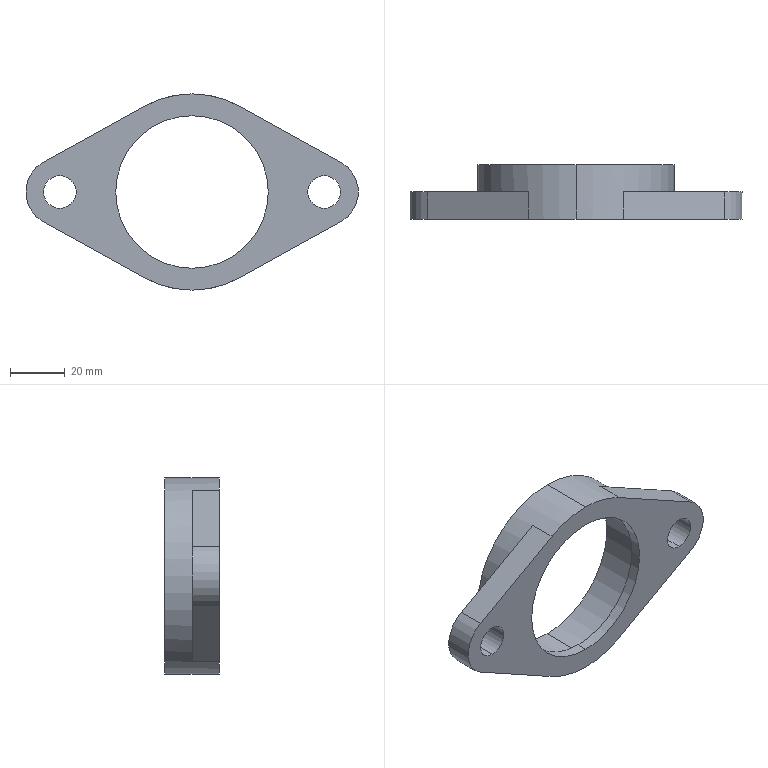Part | SolidWorks | features ICE 3, Extrusion 1 | 1 solid | 21 faces | box 122 x 20 x 72 mm | volume 37889 mm3 | cylinder 12 | plane 9 | commonest cylinder face diameters 12 x4 25 x2 56 x2 62 x2 72 x2
STEP:
#1=CARTESIAN_POINT('',(0.,0.,-28.));
#2=VERTEX_POINT('',#1);
#3=CARTESIAN_POINT('',(0.,0.,28.));
#4=VERTEX_POINT('',#3);
#5=CARTESIAN_POINT('',(0.,0.,0.));
#6=DIRECTION('',(0.,1.,0.));
#7=DIRECTION('',(0.,0.,1.));
#8=AXIS2_PLACEMENT_3D('',#5,#6,#7);
#9=CIRCLE('',#8,28.);
#10=EDGE_CURVE('',#2,#4,#9,.T.);
#11=ORIENTED_EDGE('',*,*,#10,.F.);
#12=CARTESIAN_POINT('',(0.,4.,-28.));
#13=VERTEX_POINT('',#12);
#14=CARTESIAN_POINT('',(0.,-12.,-28.));
#15=DIRECTION('',(0.,1.,0.));
#16=VECTOR('',#15,1000.);
#17=LINE('',#14,#16);
#18=EDGE_CURVE('',#2,#13,#17,.T.);
#19=ORIENTED_EDGE('',*,*,#18,.T.);
#20=CARTESIAN_POINT('',(0.,4.,28.));
#21=VERTEX_POINT('',#20);
#22=CARTESIAN_POINT('',(0.,4.,0.));
#23=DIRECTION('',(0.,1.,0.));
#24=DIRECTION('',(0.,0.,1.));
#25=AXIS2_PLACEMENT_3D('',#22,#23,#24);
#26=CIRCLE('',#25,28.);
#27=EDGE_CURVE('',#13,#21,#26,.T.);
#28=ORIENTED_EDGE('',*,*,#27,.T.);
#29=CARTESIAN_POINT('',(0.,-12.,28.));
#30=DIRECTION('',(0.,1.,0.));
#31=VECTOR('',#30,1000.);
#32=LINE('',#29,#31);
#33=EDGE_CURVE('',#4,#21,#32,.T.);
#34=ORIENTED_EDGE('',*,*,#33,.F.);
#35=EDGE_LOOP('',(#11,#19,#28,#34));
#36=FACE_OUTER_BOUND('',#35,.T.);
#37=CARTESIAN_POINT('',(0.,-12.,0.));
#38=DIRECTION('',(0.,1.,0.));
#39=DIRECTION('',(0.,0.,1.));
#40=AXIS2_PLACEMENT_3D('',#37,#38,#39);
#41=CYLINDRICAL_SURFACE('',#40,28.);
#42=ADVANCED_FACE('',(#36),#41,.F.);
#43=CARTESIAN_POINT('',(0.,4.,-31.));
#44=VERTEX_POINT('',#43);
#45=CARTESIAN_POINT('',(0.,4.,31.));
#46=VERTEX_POINT('',#45);
#47=CARTESIAN_POINT('',(0.,4.,0.));
#48=DIRECTION('',(0.,1.,0.));
#49=DIRECTION('',(0.,0.,1.));
#50=AXIS2_PLACEMENT_3D('',#47,#48,#49);
#51=CIRCLE('',#50,31.);
#52=EDGE_CURVE('',#44,#46,#51,.T.);
#53=ORIENTED_EDGE('',*,*,#52,.F.);
#54=CARTESIAN_POINT('',(0.,20.,-31.));
#55=VERTEX_POINT('',#54);
#56=CARTESIAN_POINT('',(0.,4.,-31.));
#57=DIRECTION('',(0.,1.,0.));
#58=VECTOR('',#57,1000.);
#59=LINE('',#56,#58);
#60=EDGE_CURVE('',#44,#55,#59,.T.);
#61=ORIENTED_EDGE('',*,*,#60,.T.);
#62=CARTESIAN_POINT('',(0.,20.,31.));
#63=VERTEX_POINT('',#62);
#64=CARTESIAN_POINT('',(0.,20.,0.));
#65=DIRECTION('',(0.,1.,0.));
#66=DIRECTION('',(0.,0.,1.));
#67=AXIS2_PLACEMENT_3D('',#64,#65,#66);
#68=CIRCLE('',#67,31.);
#69=EDGE_CURVE('',#55,#63,#68,.T.);
#70=ORIENTED_EDGE('',*,*,#69,.T.);
#71=CARTESIAN_POINT('',(0.,4.,31.));
#72=DIRECTION('',(0.,1.,0.));
#73=VECTOR('',#72,1000.);
#74=LINE('',#71,#73);
#75=EDGE_CURVE('',#46,#63,#74,.T.);
#76=ORIENTED_EDGE('',*,*,#75,.F.);
#77=EDGE_LOOP('',(#53,#61,#70,#76));
#78=FACE_OUTER_BOUND('',#77,.T.);
#79=CARTESIAN_POINT('',(0.,4.,0.));
#80=DIRECTION('',(0.,1.,0.));
#81=DIRECTION('',(0.,0.,1.));
#82=AXIS2_PLACEMENT_3D('',#79,#80,#81);
#83=CYLINDRICAL_SURFACE('',#82,31.);
#84=ADVANCED_FACE('',(#78),#83,.F.);
#85=CARTESIAN_POINT('',(-48.5,10.,-6.));
#86=VERTEX_POINT('',#85);
#87=CARTESIAN_POINT('',(-48.5,10.,6.));
#88=VERTEX_POINT('',#87);
#89=CARTESIAN_POINT('',(-48.5,10.,0.));
#90=DIRECTION('',(0.,1.,0.));
#91=DIRECTION('',(0.,0.,1.));
#92=AXIS2_PLACEMENT_3D('',#89,#90,#91);
#93=CIRCLE('',#92,6.);
#94=EDGE_CURVE('',#86,#88,#93,.T.);
#95=ORIENTED_EDGE('',*,*,#94,.T.);
#96=CARTESIAN_POINT('',(-48.5,0.,6.));
#97=VERTEX_POINT('',#96);
#98=CARTESIAN_POINT('',(-48.5,10.,6.));
#99=DIRECTION('',(0.,-1.,0.));
#100=VECTOR('',#99,1000.);
#101=LINE('',#98,#100);
#102=EDGE_CURVE('',#88,#97,#101,.T.);
#103=ORIENTED_EDGE('',*,*,#102,.T.);
#104=CARTESIAN_POINT('',(-48.5,0.,-6.));
#105=VERTEX_POINT('',#104);
#106=CARTESIAN_POINT('',(-48.5,0.,0.));
#107=DIRECTION('',(0.,1.,0.));
#108=DIRECTION('',(0.,0.,1.));
#109=AXIS2_PLACEMENT_3D('',#106,#107,#108);
#110=CIRCLE('',#109,6.);
#111=EDGE_CURVE('',#105,#97,#110,.T.);
#112=ORIENTED_EDGE('',*,*,#111,.F.);
#113=CARTESIAN_POINT('',(-48.5,10.,-6.));
#114=DIRECTION('',(0.,-1.,0.));
#115=VECTOR('',#114,1000.);
#116=LINE('',#113,#115);
#117=EDGE_CURVE('',#86,#105,#116,.T.);
#118=ORIENTED_EDGE('',*,*,#117,.F.);
#119=EDGE_LOOP('',(#95,#103,#112,#118));
#120=FACE_OUTER_BOUND('',#119,.T.);
#121=CARTESIAN_POINT('',(-48.5,10.,0.));
#122=DIRECTION('',(0.,-1.,0.));
#123=DIRECTION('',(0.,0.,-1.));
#124=AXIS2_PLACEMENT_3D('',#121,#122,#123);
#125=CYLINDRICAL_SURFACE('',#124,6.);
#126=ADVANCED_FACE('',(#120),#125,.F.);
#127=CARTESIAN_POINT('',(48.5,10.,-6.));
#128=VERTEX_POINT('',#127);
#129=CARTESIAN_POINT('',(48.5,10.,6.));
#130=VERTEX_POINT('',#129);
#131=CARTESIAN_POINT('',(48.5,10.,0.));
#132=DIRECTION('',(0.,1.,0.));
#133=DIRECTION('',(0.,0.,1.));
#134=AXIS2_PLACEMENT_3D('',#131,#132,#133);
#135=CIRCLE('',#134,6.);
#136=EDGE_CURVE('',#128,#130,#135,.T.);
#137=ORIENTED_EDGE('',*,*,#136,.T.);
#138=CARTESIAN_POINT('',(48.5,0.,6.));
#139=VERTEX_POINT('',#138);
#140=CARTESIAN_POINT('',(48.5,10.,6.));
#141=DIRECTION('',(0.,-1.,0.));
#142=VECTOR('',#141,1000.);
#143=LINE('',#140,#142);
#144=EDGE_CURVE('',#130,#139,#143,.T.);
#145=ORIENTED_EDGE('',*,*,#144,.T.);
#146=CARTESIAN_POINT('',(48.5,0.,-6.));
#147=VERTEX_POINT('',#146);
#148=CARTESIAN_POINT('',(48.5,0.,0.));
#149=DIRECTION('',(0.,1.,0.));
#150=DIRECTION('',(0.,0.,1.));
#151=AXIS2_PLACEMENT_3D('',#148,#149,#150);
#152=CIRCLE('',#151,6.);
#153=EDGE_CURVE('',#147,#139,#152,.T.);
#154=ORIENTED_EDGE('',*,*,#153,.F.);
#155=CARTESIAN_POINT('',(48.5,10.,-6.));
#156=DIRECTION('',(0.,-1.,0.));
#157=VECTOR('',#156,1000.);
#158=LINE('',#155,#157);
#159=EDGE_CURVE('',#128,#147,#158,.T.);
#160=ORIENTED_EDGE('',*,*,#159,.F.);
#161=EDGE_LOOP('',(#137,#145,#154,#160));
#162=FACE_OUTER_BOUND('',#161,.T.);
#163=CARTESIAN_POINT('',(48.5,10.,0.));
#164=DIRECTION('',(0.,-1.,0.));
#165=DIRECTION('',(0.,0.,-1.));
#166=AXIS2_PLACEMENT_3D('',#163,#164,#165);
#167=CYLINDRICAL_SURFACE('',#166,6.);
#168=ADVANCED_FACE('',(#162),#167,.F.);
#169=CARTESIAN_POINT('',(0.,20.,36.));
#170=VERTEX_POINT('',#169);
#171=CARTESIAN_POINT('',(0.,20.,-36.));
#172=VERTEX_POINT('',#171);
#173=CARTESIAN_POINT('',(0.,20.,0.));
#174=DIRECTION('',(0.,1.,0.));
#175=DIRECTION('',(0.,0.,1.));
#176=AXIS2_PLACEMENT_3D('',#173,#174,#175);
#177=CIRCLE('',#176,36.);
#178=EDGE_CURVE('',#170,#172,#177,.T.);
#179=ORIENTED_EDGE('',*,*,#178,.F.);
#180=CARTESIAN_POINT('',(0.,0.,36.));
#181=VERTEX_POINT('',#180);
#182=CARTESIAN_POINT('',(0.,10.,36.));
#183=DIRECTION('',(0.,-1.,0.));
#184=VECTOR('',#183,1000.);
#185=LINE('',#182,#184);
#186=EDGE_CURVE('',#170,#181,#185,.T.);
#187=ORIENTED_EDGE('',*,*,#186,.T.);
#188=CARTESIAN_POINT('',(17.443,0.,31.492));
#189=VERTEX_POINT('',#188);
#190=CARTESIAN_POINT('',(0.,0.,0.));
#191=DIRECTION('',(0.,1.,0.));
#192=DIRECTION('',(0.,0.,1.));
#193=AXIS2_PLACEMENT_3D('',#190,#191,#192);
#194=CIRCLE('',#193,36.);
#195=EDGE_CURVE('',#181,#189,#194,.T.);
#196=ORIENTED_EDGE('',*,*,#195,.T.);
#197=CARTESIAN_POINT('',(17.443,10.,31.492));
#198=VERTEX_POINT('',#197);
#199=CARTESIAN_POINT('',(17.443,10.,31.492));
#200=DIRECTION('',(0.,-1.,0.));
#201=VECTOR('',#200,1000.);
#202=LINE('',#199,#201);
#203=EDGE_CURVE('',#198,#189,#202,.T.);
#204=ORIENTED_EDGE('',*,*,#203,.F.);
#205=CARTESIAN_POINT('',(17.443,10.,-31.492));
#206=VERTEX_POINT('',#205);
#207=CARTESIAN_POINT('',(0.,10.,0.));
#208=DIRECTION('',(0.,1.,0.));
#209=DIRECTION('',(0.,0.,1.));
#210=AXIS2_PLACEMENT_3D('',#207,#208,#209);
#211=CIRCLE('',#210,36.);
#212=EDGE_CURVE('',#198,#206,#211,.T.);
#213=ORIENTED_EDGE('',*,*,#212,.T.);
#214=CARTESIAN_POINT('',(17.443,0.,-31.492));
#215=VERTEX_POINT('',#214);
#216=CARTESIAN_POINT('',(17.443,10.,-31.492));
#217=DIRECTION('',(0.,-1.,0.));
#218=VECTOR('',#217,1000.);
#219=LINE('',#216,#218);
#220=EDGE_CURVE('',#206,#215,#219,.T.);
#221=ORIENTED_EDGE('',*,*,#220,.T.);
#222=CARTESIAN_POINT('',(0.,0.,-36.));
#223=VERTEX_POINT('',#222);
#224=CARTESIAN_POINT('',(0.,0.,0.));
#225=DIRECTION('',(0.,1.,0.));
#226=DIRECTION('',(0.,0.,1.));
#227=AXIS2_PLACEMENT_3D('',#224,#225,#226);
#228=CIRCLE('',#227,36.);
#229=EDGE_CURVE('',#215,#223,#228,.T.);
#230=ORIENTED_EDGE('',*,*,#229,.T.);
#231=CARTESIAN_POINT('',(0.,10.,-36.));
#232=DIRECTION('',(0.,-1.,0.));
#233=VECTOR('',#232,1000.);
#234=LINE('',#231,#233);
#235=EDGE_CURVE('',#172,#223,#234,.T.);
#236=ORIENTED_EDGE('',*,*,#235,.F.);
#237=EDGE_LOOP('',(#179,#187,#196,#204,#213,#221,#230,#236));
#238=FACE_OUTER_BOUND('',#237,.T.);
#239=CARTESIAN_POINT('',(0.,10.,0.));
#240=DIRECTION('',(0.,-1.,0.));
#241=DIRECTION('',(0.,0.,-1.));
#242=AXIS2_PLACEMENT_3D('',#239,#240,#241);
#243=CYLINDRICAL_SURFACE('',#242,36.);
#244=ADVANCED_FACE('',(#238),#243,.T.);
#245=ORIENTED_EDGE('',*,*,#212,.F.);
#246=CARTESIAN_POINT('',(54.557,10.,10.935));
#247=VERTEX_POINT('',#246);
#248=CARTESIAN_POINT('',(54.557,10.,10.935));
#249=DIRECTION('',(0.8748,0.,-0.4845));
#250=VECTOR('',#249,1000.);
#251=LINE('',#248,#250);
#252=EDGE_CURVE('',#198,#247,#251,.T.);
#253=ORIENTED_EDGE('',*,*,#252,.T.);
#254=CARTESIAN_POINT('',(54.557,10.,-10.935));
#255=VERTEX_POINT('',#254);
#256=CARTESIAN_POINT('',(48.5,10.,0.));
#257=DIRECTION('',(0.,1.,0.));
#258=DIRECTION('',(0.,0.,1.));
#259=AXIS2_PLACEMENT_3D('',#256,#257,#258);
#260=CIRCLE('',#259,12.5);
#261=EDGE_CURVE('',#247,#255,#260,.T.);
#262=ORIENTED_EDGE('',*,*,#261,.T.);
#263=CARTESIAN_POINT('',(17.443,10.,-31.492));
#264=DIRECTION('',(-0.8748,0.,-0.4845));
#265=VECTOR('',#264,1000.);
#266=LINE('',#263,#265);
#267=EDGE_CURVE('',#255,#206,#266,.T.);
#268=ORIENTED_EDGE('',*,*,#267,.T.);
#269=EDGE_LOOP('',(#245,#253,#262,#268));
#270=FACE_OUTER_BOUND('',#269,.T.);
#271=ORIENTED_EDGE('',*,*,#136,.F.);
#272=CARTESIAN_POINT('',(48.5,10.,0.));
#273=DIRECTION('',(0.,1.,0.));
#274=DIRECTION('',(0.,0.,1.));
#275=AXIS2_PLACEMENT_3D('',#272,#273,#274);
#276=CIRCLE('',#275,6.);
#277=EDGE_CURVE('',#130,#128,#276,.T.);
#278=ORIENTED_EDGE('',*,*,#277,.F.);
#279=EDGE_LOOP('',(#271,#278));
#280=FACE_BOUND('',#279,.T.);
#281=CARTESIAN_POINT('',(-48.5,10.,0.));
#282=DIRECTION('',(0.,1.,0.));
#283=DIRECTION('',(0.,0.,1.));
#284=AXIS2_PLACEMENT_3D('',#281,#282,#283);
#285=PLANE('',#284);
#286=ADVANCED_FACE('',(#270,#280),#285,.T.);
#287=CARTESIAN_POINT('',(-17.443,10.,-31.492));
#288=VERTEX_POINT('',#287);
#289=CARTESIAN_POINT('',(-17.443,10.,31.492));
#290=VERTEX_POINT('',#289);
#291=CARTESIAN_POINT('',(0.,10.,0.));
#292=DIRECTION('',(0.,1.,0.));
#293=DIRECTION('',(0.,0.,1.));
#294=AXIS2_PLACEMENT_3D('',#291,#292,#293);
#295=CIRCLE('',#294,36.);
#296=EDGE_CURVE('',#288,#290,#295,.T.);
#297=ORIENTED_EDGE('',*,*,#296,.F.);
#298=CARTESIAN_POINT('',(-54.557,10.,-10.935));
#299=VERTEX_POINT('',#298);
#300=CARTESIAN_POINT('',(-54.557,10.,-10.935));
#301=DIRECTION('',(-0.8748,0.,0.4845));
#302=VECTOR('',#301,1000.);
#303=LINE('',#300,#302);
#304=EDGE_CURVE('',#288,#299,#303,.T.);
#305=ORIENTED_EDGE('',*,*,#304,.T.);
#306=CARTESIAN_POINT('',(-54.557,10.,10.935));
#307=VERTEX_POINT('',#306);
#308=CARTESIAN_POINT('',(-48.5,10.,0.));
#309=DIRECTION('',(0.,1.,0.));
#310=DIRECTION('',(0.,0.,1.));
#311=AXIS2_PLACEMENT_3D('',#308,#309,#310);
#312=CIRCLE('',#311,12.5);
#313=EDGE_CURVE('',#299,#307,#312,.T.);
#314=ORIENTED_EDGE('',*,*,#313,.T.);
#315=CARTESIAN_POINT('',(-17.443,10.,31.492));
#316=DIRECTION('',(0.8748,0.,0.4845));
#317=VECTOR('',#316,1000.);
#318=LINE('',#315,#317);
#319=EDGE_CURVE('',#307,#290,#318,.T.);
#320=ORIENTED_EDGE('',*,*,#319,.T.);
#321=EDGE_LOOP('',(#297,#305,#314,#320));
#322=FACE_OUTER_BOUND('',#321,.T.);
#323=ORIENTED_EDGE('',*,*,#94,.F.);
#324=CARTESIAN_POINT('',(-48.5,10.,0.));
#325=DIRECTION('',(0.,1.,0.));
#326=DIRECTION('',(0.,0.,1.));
#327=AXIS2_PLACEMENT_3D('',#324,#325,#326);
#328=CIRCLE('',#327,6.);
#329=EDGE_CURVE('',#88,#86,#328,.T.);
#330=ORIENTED_EDGE('',*,*,#329,.F.);
#331=EDGE_LOOP('',(#323,#330));
#332=FACE_BOUND('',#331,.T.);
#333=CARTESIAN_POINT('',(-48.5,10.,0.));
#334=DIRECTION('',(0.,1.,0.));
#335=DIRECTION('',(0.,0.,1.));
#336=AXIS2_PLACEMENT_3D('',#333,#334,#335);
#337=PLANE('',#336);
#338=ADVANCED_FACE('',(#322,#332),#337,.T.);
#339=CARTESIAN_POINT('',(0.,0.,0.));
#340=DIRECTION('',(0.,1.,0.));
#341=DIRECTION('',(0.,0.,1.));
#342=AXIS2_PLACEMENT_3D('',#339,#340,#341);
#343=CIRCLE('',#342,28.);
#344=EDGE_CURVE('',#4,#2,#343,.T.);
#345=ORIENTED_EDGE('',*,*,#344,.T.);
#346=ORIENTED_EDGE('',*,*,#10,.T.);
#347=EDGE_LOOP('',(#345,#346));
#348=FACE_BOUND('',#347,.T.);
#349=ORIENTED_EDGE('',*,*,#153,.T.);
#350=CARTESIAN_POINT('',(48.5,0.,0.));
#351=DIRECTION('',(0.,1.,0.));
#352=DIRECTION('',(0.,0.,1.));
#353=AXIS2_PLACEMENT_3D('',#350,#351,#352);
#354=CIRCLE('',#353,6.);
#355=EDGE_CURVE('',#139,#147,#354,.T.);
#356=ORIENTED_EDGE('',*,*,#355,.T.);
#357=EDGE_LOOP('',(#349,#356));
#358=FACE_BOUND('',#357,.T.);
#359=CARTESIAN_POINT('',(-54.557,0.,-10.935));
#360=VERTEX_POINT('',#359);
#361=CARTESIAN_POINT('',(-54.557,0.,10.935));
#362=VERTEX_POINT('',#361);
#363=CARTESIAN_POINT('',(-48.5,0.,0.));
#364=DIRECTION('',(0.,1.,0.));
#365=DIRECTION('',(0.,0.,1.));
#366=AXIS2_PLACEMENT_3D('',#363,#364,#365);
#367=CIRCLE('',#366,12.5);
#368=EDGE_CURVE('',#360,#362,#367,.T.);
#369=ORIENTED_EDGE('',*,*,#368,.F.);
#370=CARTESIAN_POINT('',(-17.443,0.,-31.492));
#371=VERTEX_POINT('',#370);
#372=CARTESIAN_POINT('',(-54.557,0.,-10.935));
#373=DIRECTION('',(-0.8748,0.,0.4845));
#374=VECTOR('',#373,1000.);
#375=LINE('',#372,#374);
#376=EDGE_CURVE('',#371,#360,#375,.T.);
#377=ORIENTED_EDGE('',*,*,#376,.F.);
#378=CARTESIAN_POINT('',(0.,0.,0.));
#379=DIRECTION('',(0.,1.,0.));
#380=DIRECTION('',(0.,0.,1.));
#381=AXIS2_PLACEMENT_3D('',#378,#379,#380);
#382=CIRCLE('',#381,36.);
#383=EDGE_CURVE('',#223,#371,#382,.T.);
#384=ORIENTED_EDGE('',*,*,#383,.F.);
#385=ORIENTED_EDGE('',*,*,#229,.F.);
#386=CARTESIAN_POINT('',(54.557,0.,-10.935));
#387=VERTEX_POINT('',#386);
#388=CARTESIAN_POINT('',(17.443,0.,-31.492));
#389=DIRECTION('',(-0.8748,0.,-0.4845));
#390=VECTOR('',#389,1000.);
#391=LINE('',#388,#390);
#392=EDGE_CURVE('',#387,#215,#391,.T.);
#393=ORIENTED_EDGE('',*,*,#392,.F.);
#394=CARTESIAN_POINT('',(54.557,0.,10.935));
#395=VERTEX_POINT('',#394);
#396=CARTESIAN_POINT('',(48.5,0.,0.));
#397=DIRECTION('',(0.,1.,0.));
#398=DIRECTION('',(0.,0.,1.));
#399=AXIS2_PLACEMENT_3D('',#396,#397,#398);
#400=CIRCLE('',#399,12.5);
#401=EDGE_CURVE('',#395,#387,#400,.T.);
#402=ORIENTED_EDGE('',*,*,#401,.F.);
#403=CARTESIAN_POINT('',(54.557,0.,10.935));
#404=DIRECTION('',(0.8748,0.,-0.4845));
#405=VECTOR('',#404,1000.);
#406=LINE('',#403,#405);
#407=EDGE_CURVE('',#189,#395,#406,.T.);
#408=ORIENTED_EDGE('',*,*,#407,.F.);
#409=ORIENTED_EDGE('',*,*,#195,.F.);
#410=CARTESIAN_POINT('',(-17.443,0.,31.492));
#411=VERTEX_POINT('',#410);
#412=CARTESIAN_POINT('',(0.,0.,0.));
#413=DIRECTION('',(0.,1.,0.));
#414=DIRECTION('',(0.,0.,1.));
#415=AXIS2_PLACEMENT_3D('',#412,#413,#414);
#416=CIRCLE('',#415,36.);
#417=EDGE_CURVE('',#411,#181,#416,.T.);
#418=ORIENTED_EDGE('',*,*,#417,.F.);
#419=CARTESIAN_POINT('',(-17.443,0.,31.492));
#420=DIRECTION('',(0.8748,0.,0.4845));
#421=VECTOR('',#420,1000.);
#422=LINE('',#419,#421);
#423=EDGE_CURVE('',#362,#411,#422,.T.);
#424=ORIENTED_EDGE('',*,*,#423,.F.);
#425=EDGE_LOOP('',(#369,#377,#384,#385,#393,#402,#408,#409,#418,#424));
#426=FACE_OUTER_BOUND('',#425,.T.);
#427=ORIENTED_EDGE('',*,*,#111,.T.);
#428=CARTESIAN_POINT('',(-48.5,0.,0.));
#429=DIRECTION('',(0.,1.,0.));
#430=DIRECTION('',(0.,0.,1.));
#431=AXIS2_PLACEMENT_3D('',#428,#429,#430);
#432=CIRCLE('',#431,6.);
#433=EDGE_CURVE('',#97,#105,#432,.T.);
#434=ORIENTED_EDGE('',*,*,#433,.T.);
#435=EDGE_LOOP('',(#427,#434));
#436=FACE_BOUND('',#435,.T.);
#437=CARTESIAN_POINT('',(-48.5,0.,0.));
#438=DIRECTION('',(0.,1.,0.));
#439=DIRECTION('',(0.,0.,1.));
#440=AXIS2_PLACEMENT_3D('',#437,#438,#439);
#441=PLANE('',#440);
#442=ADVANCED_FACE('',(#348,#358,#426,#436),#441,.F.);
#443=ORIENTED_EDGE('',*,*,#368,.T.);
#444=CARTESIAN_POINT('',(-54.557,10.,10.935));
#445=DIRECTION('',(0.,-1.,0.));
#446=VECTOR('',#445,1000.);
#447=LINE('',#444,#446);
#448=EDGE_CURVE('',#307,#362,#447,.T.);
#449=ORIENTED_EDGE('',*,*,#448,.F.);
#450=ORIENTED_EDGE('',*,*,#313,.F.);
#451=CARTESIAN_POINT('',(-54.557,10.,-10.935));
#452=DIRECTION('',(0.,-1.,0.));
#453=VECTOR('',#452,1000.);
#454=LINE('',#451,#453);
#455=EDGE_CURVE('',#299,#360,#454,.T.);
#456=ORIENTED_EDGE('',*,*,#455,.T.);
#457=EDGE_LOOP('',(#443,#449,#450,#456));
#458=FACE_OUTER_BOUND('',#457,.T.);
#459=CARTESIAN_POINT('',(-48.5,10.,0.));
#460=DIRECTION('',(0.,-1.,0.));
#461=DIRECTION('',(0.,0.,-1.));
#462=AXIS2_PLACEMENT_3D('',#459,#460,#461);
#463=CYLINDRICAL_SURFACE('',#462,12.5);
#464=ADVANCED_FACE('',(#458),#463,.T.);
#465=ORIENTED_EDGE('',*,*,#423,.T.);
#466=CARTESIAN_POINT('',(-17.443,10.,31.492));
#467=DIRECTION('',(0.,-1.,0.));
#468=VECTOR('',#467,1000.);
#469=LINE('',#466,#468);
#470=EDGE_CURVE('',#290,#411,#469,.T.);
#471=ORIENTED_EDGE('',*,*,#470,.F.);
#472=ORIENTED_EDGE('',*,*,#319,.F.);
#473=ORIENTED_EDGE('',*,*,#448,.T.);
#474=EDGE_LOOP('',(#465,#471,#472,#473));
#475=FACE_OUTER_BOUND('',#474,.T.);
#476=CARTESIAN_POINT('',(-17.443,10.,31.492));
#477=DIRECTION('',(0.4845,0.,-0.8748));
#478=DIRECTION('',(-0.8748,0.,-0.4845));
#479=AXIS2_PLACEMENT_3D('',#476,#477,#478);
#480=PLANE('',#479);
#481=ADVANCED_FACE('',(#475),#480,.F.);
#482=ORIENTED_EDGE('',*,*,#407,.T.);
#483=CARTESIAN_POINT('',(54.557,10.,10.935));
#484=DIRECTION('',(0.,-1.,0.));
#485=VECTOR('',#484,1000.);
#486=LINE('',#483,#485);
#487=EDGE_CURVE('',#247,#395,#486,.T.);
#488=ORIENTED_EDGE('',*,*,#487,.F.);
#489=ORIENTED_EDGE('',*,*,#252,.F.);
#490=ORIENTED_EDGE('',*,*,#203,.T.);
#491=EDGE_LOOP('',(#482,#488,#489,#490));
#492=FACE_OUTER_BOUND('',#491,.T.);
#493=CARTESIAN_POINT('',(54.557,10.,10.935));
#494=DIRECTION('',(-0.4845,0.,-0.8748));
#495=DIRECTION('',(-0.8748,0.,0.4845));
#496=AXIS2_PLACEMENT_3D('',#493,#494,#495);
#497=PLANE('',#496);
#498=ADVANCED_FACE('',(#492),#497,.F.);
#499=ORIENTED_EDGE('',*,*,#401,.T.);
#500=CARTESIAN_POINT('',(54.557,10.,-10.935));
#501=DIRECTION('',(0.,-1.,0.));
#502=VECTOR('',#501,1000.);
#503=LINE('',#500,#502);
#504=EDGE_CURVE('',#255,#387,#503,.T.);
#505=ORIENTED_EDGE('',*,*,#504,.F.);
#506=ORIENTED_EDGE('',*,*,#261,.F.);
#507=ORIENTED_EDGE('',*,*,#487,.T.);
#508=EDGE_LOOP('',(#499,#505,#506,#507));
#509=FACE_OUTER_BOUND('',#508,.T.);
#510=CARTESIAN_POINT('',(48.5,10.,0.));
#511=DIRECTION('',(0.,-1.,0.));
#512=DIRECTION('',(0.,0.,-1.));
#513=AXIS2_PLACEMENT_3D('',#510,#511,#512);
#514=CYLINDRICAL_SURFACE('',#513,12.5);
#515=ADVANCED_FACE('',(#509),#514,.T.);
#516=ORIENTED_EDGE('',*,*,#392,.T.);
#517=ORIENTED_EDGE('',*,*,#220,.F.);
#518=ORIENTED_EDGE('',*,*,#267,.F.);
#519=ORIENTED_EDGE('',*,*,#504,.T.);
#520=EDGE_LOOP('',(#516,#517,#518,#519));
#521=FACE_OUTER_BOUND('',#520,.T.);
#522=CARTESIAN_POINT('',(17.443,10.,-31.492));
#523=DIRECTION('',(-0.4845,0.,0.8748));
#524=DIRECTION('',(0.8748,0.,0.4845));
#525=AXIS2_PLACEMENT_3D('',#522,#523,#524);
#526=PLANE('',#525);
#527=ADVANCED_FACE('',(#521),#526,.F.);
#528=ORIENTED_EDGE('',*,*,#186,.F.);
#529=CARTESIAN_POINT('',(0.,20.,0.));
#530=DIRECTION('',(0.,1.,0.));
#531=DIRECTION('',(0.,0.,1.));
#532=AXIS2_PLACEMENT_3D('',#529,#530,#531);
#533=CIRCLE('',#532,36.);
#534=EDGE_CURVE('',#172,#170,#533,.T.);
#535=ORIENTED_EDGE('',*,*,#534,.F.);
#536=ORIENTED_EDGE('',*,*,#235,.T.);
#537=ORIENTED_EDGE('',*,*,#383,.T.);
#538=CARTESIAN_POINT('',(-17.443,10.,-31.492));
#539=DIRECTION('',(0.,-1.,0.));
#540=VECTOR('',#539,1000.);
#541=LINE('',#538,#540);
#542=EDGE_CURVE('',#288,#371,#541,.T.);
#543=ORIENTED_EDGE('',*,*,#542,.F.);
#544=ORIENTED_EDGE('',*,*,#296,.T.);
#545=ORIENTED_EDGE('',*,*,#470,.T.);
#546=ORIENTED_EDGE('',*,*,#417,.T.);
#547=EDGE_LOOP('',(#528,#535,#536,#537,#543,#544,#545,#546));
#548=FACE_OUTER_BOUND('',#547,.T.);
#549=CARTESIAN_POINT('',(0.,10.,0.));
#550=DIRECTION('',(0.,-1.,0.));
#551=DIRECTION('',(0.,0.,-1.));
#552=AXIS2_PLACEMENT_3D('',#549,#550,#551);
#553=CYLINDRICAL_SURFACE('',#552,36.);
#554=ADVANCED_FACE('',(#548),#553,.T.);
#555=ORIENTED_EDGE('',*,*,#376,.T.);
#556=ORIENTED_EDGE('',*,*,#455,.F.);
#557=ORIENTED_EDGE('',*,*,#304,.F.);
#558=ORIENTED_EDGE('',*,*,#542,.T.);
#559=EDGE_LOOP('',(#555,#556,#557,#558));
#560=FACE_OUTER_BOUND('',#559,.T.);
#561=CARTESIAN_POINT('',(-54.557,10.,-10.935));
#562=DIRECTION('',(0.4845,0.,0.8748));
#563=DIRECTION('',(0.8748,0.,-0.4845));
#564=AXIS2_PLACEMENT_3D('',#561,#562,#563);
#565=PLANE('',#564);
#566=ADVANCED_FACE('',(#560),#565,.F.);
#567=ORIENTED_EDGE('',*,*,#144,.F.);
#568=ORIENTED_EDGE('',*,*,#277,.T.);
#569=ORIENTED_EDGE('',*,*,#159,.T.);
#570=ORIENTED_EDGE('',*,*,#355,.F.);
#571=EDGE_LOOP('',(#567,#568,#569,#570));
#572=FACE_OUTER_BOUND('',#571,.T.);
#573=CARTESIAN_POINT('',(48.5,10.,0.));
#574=DIRECTION('',(0.,-1.,0.));
#575=DIRECTION('',(0.,0.,-1.));
#576=AXIS2_PLACEMENT_3D('',#573,#574,#575);
#577=CYLINDRICAL_SURFACE('',#576,6.);
#578=ADVANCED_FACE('',(#572),#577,.F.);
#579=ORIENTED_EDGE('',*,*,#102,.F.);
#580=ORIENTED_EDGE('',*,*,#329,.T.);
#581=ORIENTED_EDGE('',*,*,#117,.T.);
#582=ORIENTED_EDGE('',*,*,#433,.F.);
#583=EDGE_LOOP('',(#579,#580,#581,#582));
#584=FACE_OUTER_BOUND('',#583,.T.);
#585=CARTESIAN_POINT('',(-48.5,10.,0.));
#586=DIRECTION('',(0.,-1.,0.));
#587=DIRECTION('',(0.,0.,-1.));
#588=AXIS2_PLACEMENT_3D('',#585,#586,#587);
#589=CYLINDRICAL_SURFACE('',#588,6.);
#590=ADVANCED_FACE('',(#584),#589,.F.);
#591=CARTESIAN_POINT('',(0.,20.,0.));
#592=DIRECTION('',(0.,1.,0.));
#593=DIRECTION('',(0.,0.,1.));
#594=AXIS2_PLACEMENT_3D('',#591,#592,#593);
#595=CIRCLE('',#594,31.);
#596=EDGE_CURVE('',#63,#55,#595,.T.);
#597=ORIENTED_EDGE('',*,*,#596,.F.);
#598=ORIENTED_EDGE('',*,*,#69,.F.);
#599=EDGE_LOOP('',(#597,#598));
#600=FACE_BOUND('',#599,.T.);
#601=ORIENTED_EDGE('',*,*,#534,.T.);
#602=ORIENTED_EDGE('',*,*,#178,.T.);
#603=EDGE_LOOP('',(#601,#602));
#604=FACE_OUTER_BOUND('',#603,.T.);
#605=CARTESIAN_POINT('',(0.,20.,0.));
#606=DIRECTION('',(0.,1.,0.));
#607=DIRECTION('',(0.,0.,1.));
#608=AXIS2_PLACEMENT_3D('',#605,#606,#607);
#609=PLANE('',#608);
#610=ADVANCED_FACE('',(#600,#604),#609,.T.);
#611=ORIENTED_EDGE('',*,*,#60,.F.);
#612=CARTESIAN_POINT('',(0.,4.,0.));
#613=DIRECTION('',(0.,1.,0.));
#614=DIRECTION('',(0.,0.,1.));
#615=AXIS2_PLACEMENT_3D('',#612,#613,#614);
#616=CIRCLE('',#615,31.);
#617=EDGE_CURVE('',#46,#44,#616,.T.);
#618=ORIENTED_EDGE('',*,*,#617,.F.);
#619=ORIENTED_EDGE('',*,*,#75,.T.);
#620=ORIENTED_EDGE('',*,*,#596,.T.);
#621=EDGE_LOOP('',(#611,#618,#619,#620));
#622=FACE_OUTER_BOUND('',#621,.T.);
#623=CARTESIAN_POINT('',(0.,4.,0.));
#624=DIRECTION('',(0.,1.,0.));
#625=DIRECTION('',(0.,0.,1.));
#626=AXIS2_PLACEMENT_3D('',#623,#624,#625);
#627=CYLINDRICAL_SURFACE('',#626,31.);
#628=ADVANCED_FACE('',(#622),#627,.F.);
#629=CARTESIAN_POINT('',(0.,4.,0.));
#630=DIRECTION('',(0.,1.,0.));
#631=DIRECTION('',(0.,0.,1.));
#632=AXIS2_PLACEMENT_3D('',#629,#630,#631);
#633=CIRCLE('',#632,28.);
#634=EDGE_CURVE('',#21,#13,#633,.T.);
#635=ORIENTED_EDGE('',*,*,#634,.F.);
#636=ORIENTED_EDGE('',*,*,#27,.F.);
#637=EDGE_LOOP('',(#635,#636));
#638=FACE_BOUND('',#637,.T.);
#639=ORIENTED_EDGE('',*,*,#617,.T.);
#640=ORIENTED_EDGE('',*,*,#52,.T.);
#641=EDGE_LOOP('',(#639,#640));
#642=FACE_OUTER_BOUND('',#641,.T.);
#643=CARTESIAN_POINT('',(0.,4.,0.));
#644=DIRECTION('',(0.,1.,0.));
#645=DIRECTION('',(0.,0.,1.));
#646=AXIS2_PLACEMENT_3D('',#643,#644,#645);
#647=PLANE('',#646);
#648=ADVANCED_FACE('',(#638,#642),#647,.T.);
#649=ORIENTED_EDGE('',*,*,#18,.F.);
#650=ORIENTED_EDGE('',*,*,#344,.F.);
#651=ORIENTED_EDGE('',*,*,#33,.T.);
#652=ORIENTED_EDGE('',*,*,#634,.T.);
#653=EDGE_LOOP('',(#649,#650,#651,#652));
#654=FACE_OUTER_BOUND('',#653,.T.);
#655=CARTESIAN_POINT('',(0.,-12.,0.));
#656=DIRECTION('',(0.,1.,0.));
#657=DIRECTION('',(0.,0.,1.));
#658=AXIS2_PLACEMENT_3D('',#655,#656,#657);
#659=CYLINDRICAL_SURFACE('',#658,28.);
#660=ADVANCED_FACE('',(#654),#659,.F.);
#661=CLOSED_SHELL('',(#42,#84,#126,#168,#244,#286,#338,#442,#464,#481,#498,#515,#527,#554,#566,#578,#590,#610,#628,#648,#660));
#662=MANIFOLD_SOLID_BREP('',#661);
#663=CARTESIAN_POINT('',(0.,0.,0.));
#664=DIRECTION('',(0.,0.,1.));
#665=DIRECTION('',(1.,0.,0.));
#666=AXIS2_PLACEMENT_3D('',#663,#664,#665);
#667=(LENGTH_UNIT()NAMED_UNIT(*)SI_UNIT(.MILLI.,.METRE.));
#668=UNCERTAINTY_MEASURE_WITH_UNIT(LENGTH_MEASURE(0.00001),#667,'','');
#669=(NAMED_UNIT(*)PLANE_ANGLE_UNIT()SI_UNIT($,.RADIAN.));
#670=(NAMED_UNIT(*)SI_UNIT($,.STERADIAN.)SOLID_ANGLE_UNIT());
#671=(GEOMETRIC_REPRESENTATION_CONTEXT(3)GLOBAL_UNCERTAINTY_ASSIGNED_CONTEXT((#668))GLOBAL_UNIT_ASSIGNED_CONTEXT((#667,#669,#670))REPRESENTATION_CONTEXT('',''));
#672=ADVANCED_BREP_SHAPE_REPRESENTATION('',(#662,#666),#671);